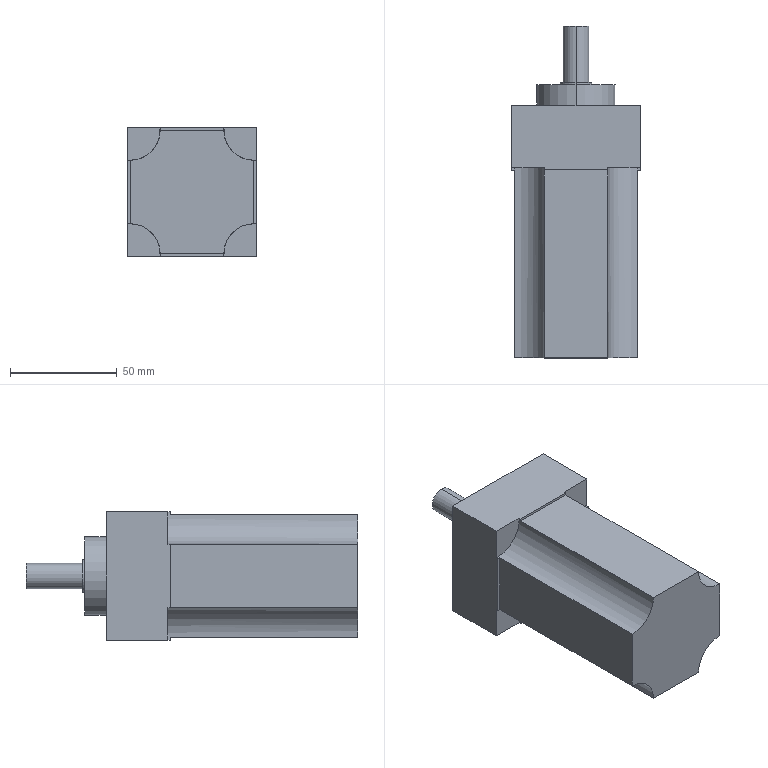Part | STEP file | PN_0007 planetary reduction stepper motor PLX60-L1-7 | 1 solid | 49 faces | box 60 x 155.5 x 60 mm | volume 360183 mm3 | plane 21 | cylinder 20 | cone 8 | commonest cylinder face diameters 4.2 x8 28 x6 12 x2 15 x2 37 x2